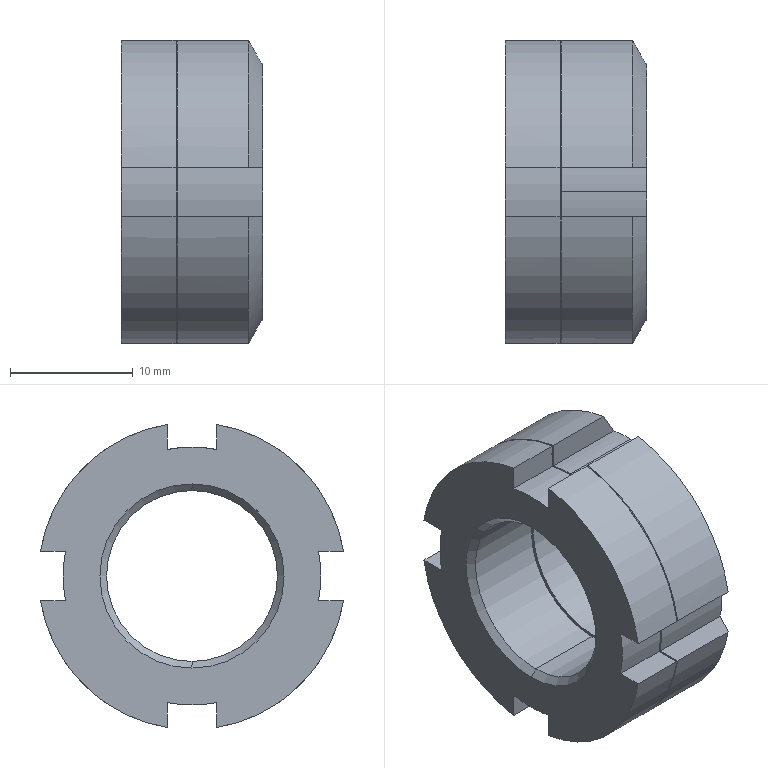Part | STEP file | 11-HLB15A11 | 1 solid | 84 faces | box 11.5 x 24.678 x 24.678 mm | volume 3349 mm3 | plane 37 | cylinder 27 | cone 20 | commonest cylinder face diameters 21 x10 25 x8 20.9 x5 13.917 x4